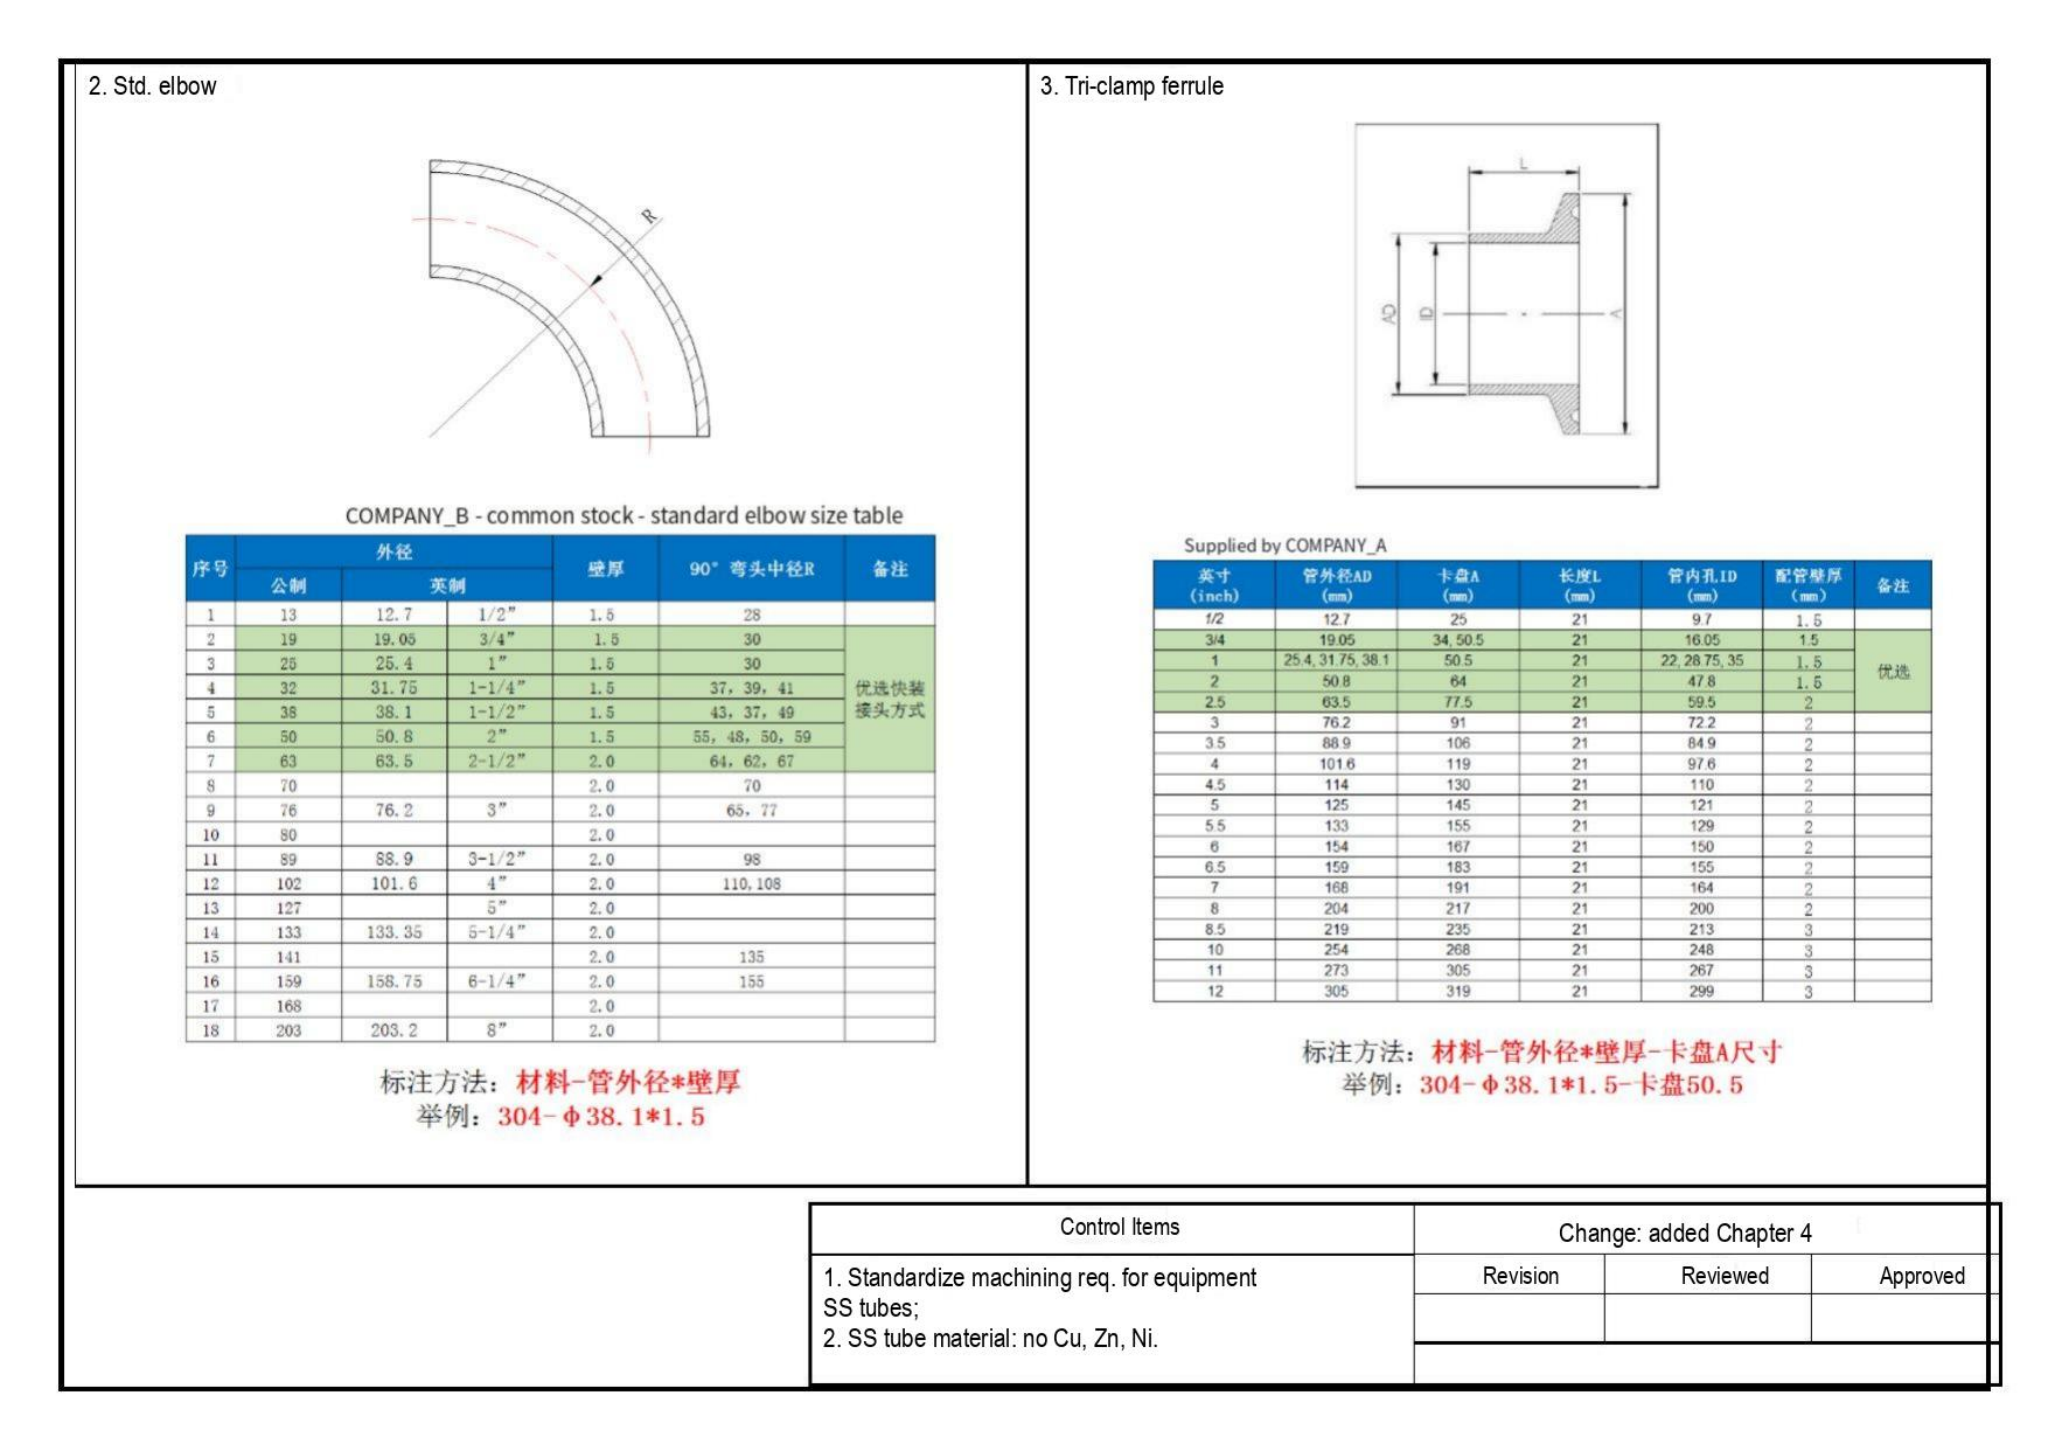2. Std. elbow

R

COMPANY_B - common stock - standard elbow size table

| 序号 | 外径 公制 | 外径 英制 | 外径 英制 | 壁厚 | 90° 弯头中径R | 备注 |
|---|---|---|---|---|---|---|
| 1 | 13 | 12.7 | 1/2" | 1.5 | 28 | |
| 2 | 19 | 19.05 | 3/4" | 1.5 | 30 | 优选快装接头方式 |
| 3 | 25 | 25.4 | 1" | 1.5 | 30 | |
| 4 | 32 | 31.75 | 1-1/4" | 1.5 | 37, 39, 41 | |
| 5 | 38 | 38.1 | 1-1/2" | 1.5 | 43, 37, 49 | |
| 6 | 50 | 50.8 | 2" | 1.5 | 55, 48, 50, 59 | |
| 7 | 63 | 63.5 | 2-1/2" | 2.0 | 64, 62, 67 | |
| 8 | 70 | | | 2.0 | 70 | |
| 9 | 76 | 76.2 | 3" | 2.0 | 65, 77 | |
| 10 | 80 | | | 2.0 | | |
| 11 | 89 | 88.9 | 3-1/2" | 2.0 | 98 | |
| 12 | 102 | 101.6 | 4" | 2.0 | 110, 108 | |
| 13 | 127 | | 5" | 2.0 | | |
| 14 | 133 | 133.35 | 5-1/4" | 2.0 | | |
| 15 | 141 | | | 2.0 | 135 | |
| 16 | 159 | 158.75 | 6-1/4" | 2.0 | 155 | |
| 17 | 168 | | | 2.0 | | |
| 18 | 203 | 203.2 | 8" | 2.0 | | |

标注方法：材料-管外径*壁厚
举例：304-Φ38.1*1.5

3. Tri-clamp ferrule

L
AD
ID
A

Supplied by COMPANY_A

| 英寸 (inch) | 管外径AD (mm) | 卡盘A (mm) | 长度L (mm) | 管内孔ID (mm) | 配管壁厚 (mm) | 备注 |
|---|---|---|---|---|---|---|
| 1/2 | 12.7 | 25 | 21 | 9.7 | 1.5 | |
| 3/4 | 19.05 | 34, 50.5 | 21 | 16.05 | 1.5 | 优选 |
| 1 | 25.4, 31.75, 38.1 | 50.5 | 21 | 22, 28.75, 35 | 1.5 | |
| 2 | 50.8 | 64 | 21 | 47.8 | 1.5 | |
| 2.5 | 63.5 | 77.5 | 21 | 59.5 | 2 | |
| 3 | 76.2 | 91 | 21 | 72.2 | 2 | |
| 3.5 | 88.9 | 106 | 21 | 84.9 | 2 | |
| 4 | 101.6 | 119 | 21 | 97.6 | 2 | |
| 4.5 | 114 | 130 | 21 | 110 | 2 | |
| 5 | 125 | 145 | 21 | 121 | 2 | |
| 5.5 | 133 | 155 | 21 | 129 | 2 | |
| 6 | 154 | 167 | 21 | 150 | 2 | |
| 6.5 | 159 | 183 | 21 | 155 | 2 | |
| 7 | 168 | 191 | 21 | 164 | 2 | |
| 8 | 204 | 217 | 21 | 200 | 2 | |
| 8.5 | 219 | 235 | 21 | 213 | 3 | |
| 10 | 254 | 268 | 21 | 248 | 3 | |
| 11 | 273 | 305 | 21 | 267 | 3 | |
| 12 | 305 | 319 | 21 | 299 | 3 | |

标注方法：材料-管外径*壁厚-卡盘A尺寸
举例：304-Φ38.1*1.5-卡盘50.5

| Control Items | Change: added Chapter 4 | | |
|---|---|---|---|
| 1. Standardize machining req. for equipment SS tubes;<br>2. SS tube material: no Cu, Zn, Ni. | Revision | Reviewed | Approved |
| | | | |
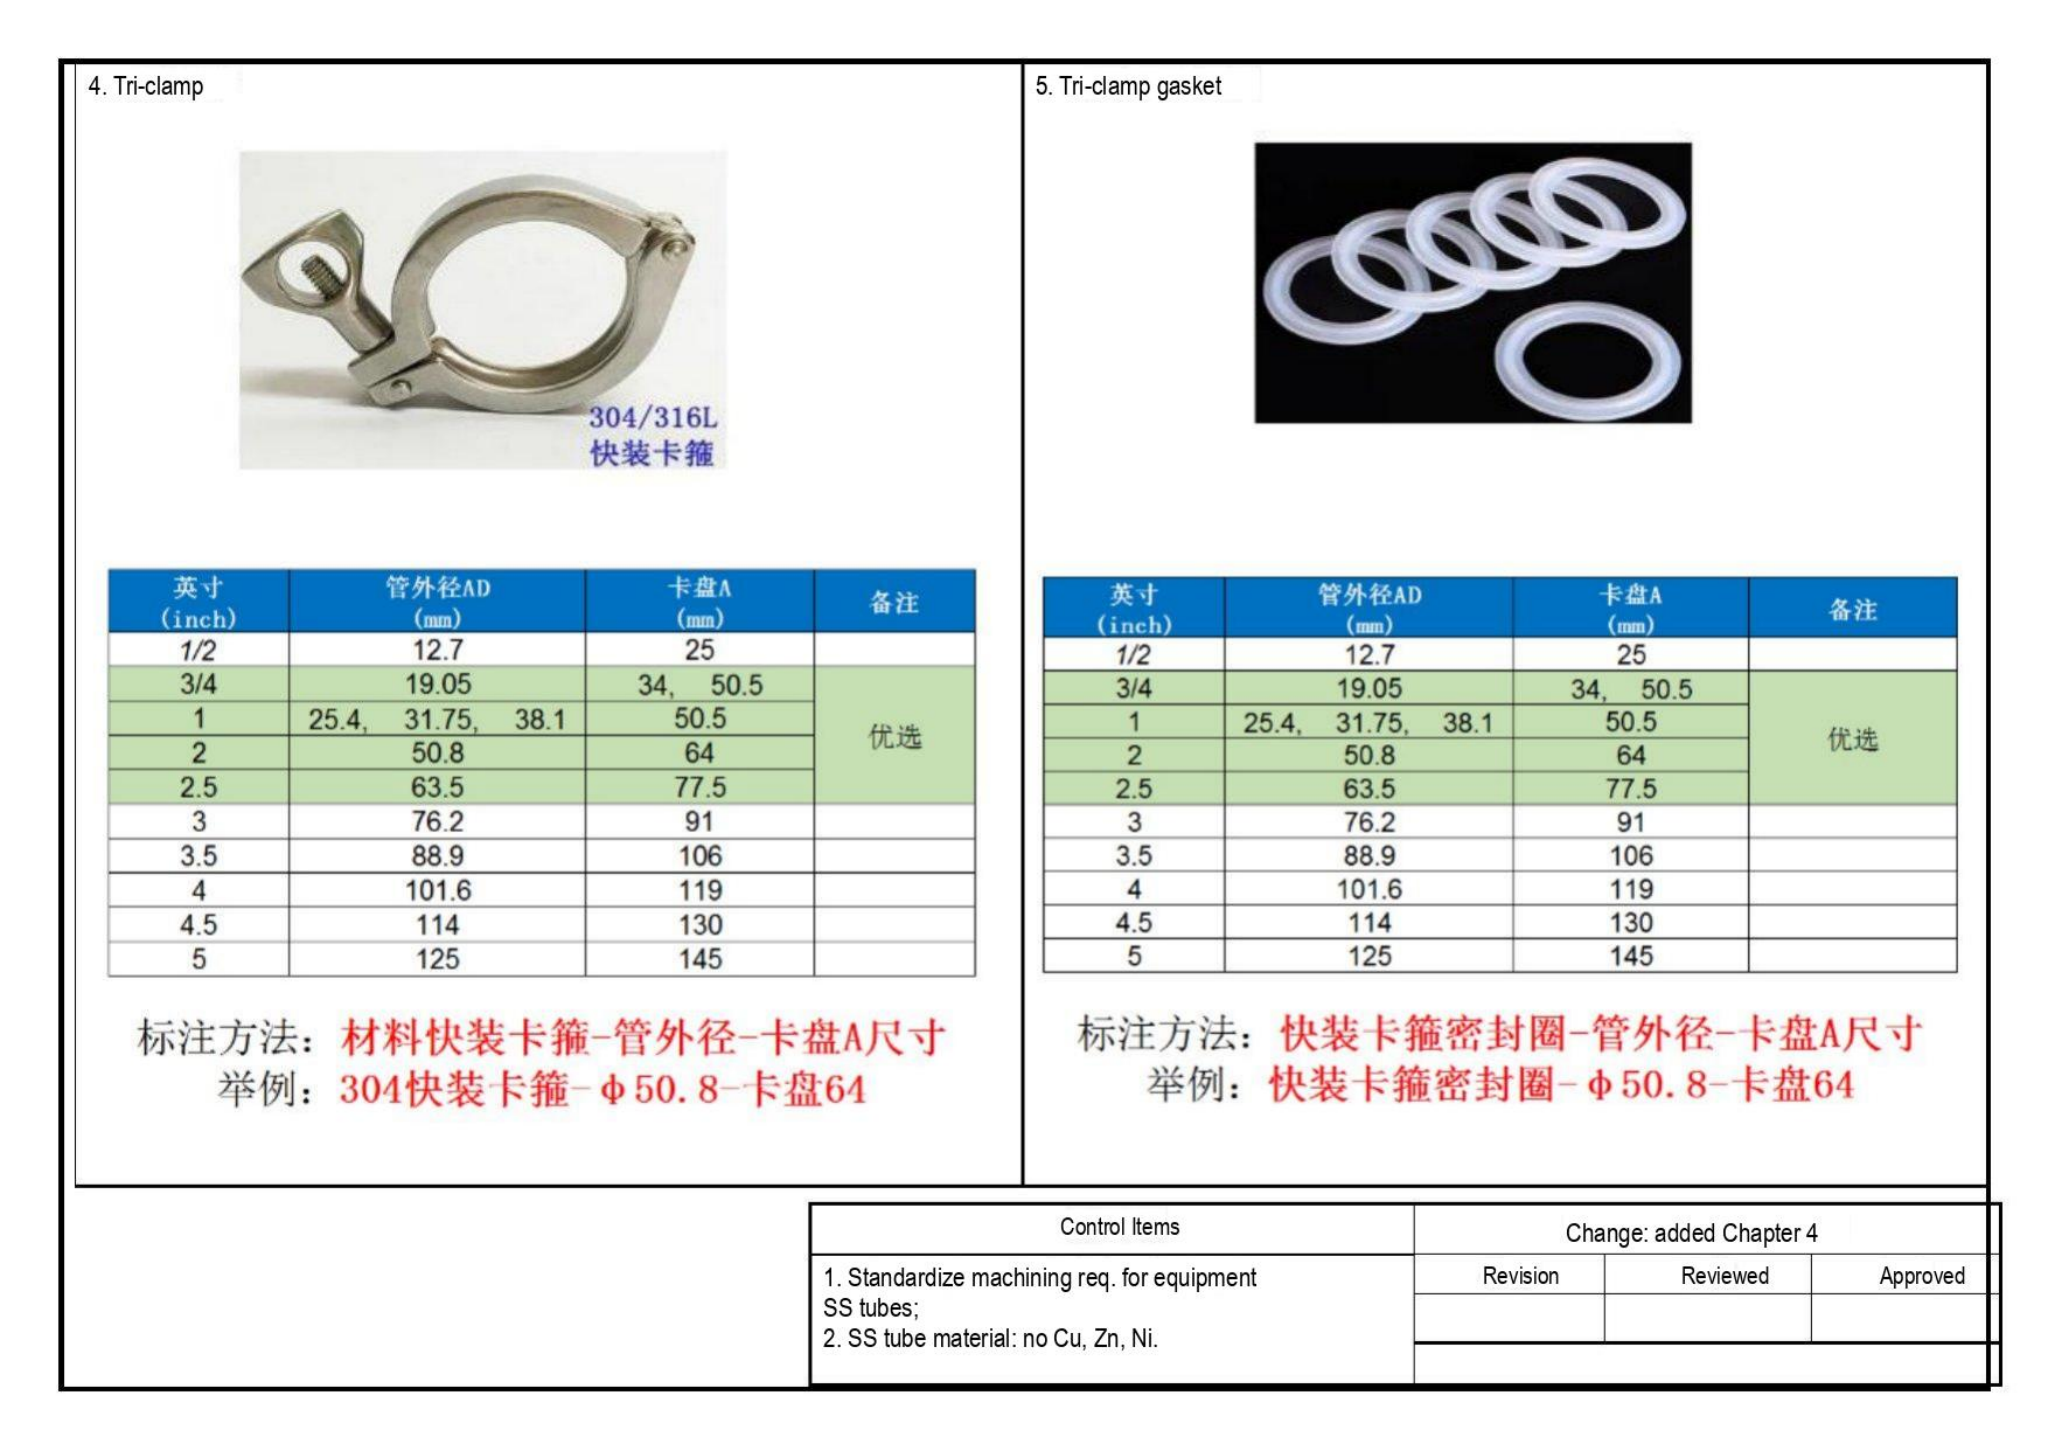4. Tri-clamp

304/316L
快装卡箍

| 英寸 (inch) | 管外径AD (mm) | 卡盘A (mm) | 备注 |
|---|---|---|---|
| 1/2 | 12.7 | 25 | |
| 3/4 | 19.05 | 34, 50.5 | 优选 |
| 1 | 25.4, 31.75, 38.1 | 50.5 | |
| 2 | 50.8 | 64 | |
| 2.5 | 63.5 | 77.5 | |
| 3 | 76.2 | 91 | |
| 3.5 | 88.9 | 106 | |
| 4 | 101.6 | 119 | |
| 4.5 | 114 | 130 | |
| 5 | 125 | 145 | |

标注方法：材料快装卡箍-管外径-卡盘A尺寸
举例：304快装卡箍-φ50.8-卡盘64

5. Tri-clamp gasket

| 英寸 (inch) | 管外径AD (mm) | 卡盘A (mm) | 备注 |
|---|---|---|---|
| 1/2 | 12.7 | 25 | |
| 3/4 | 19.05 | 34, 50.5 | 优选 |
| 1 | 25.4, 31.75, 38.1 | 50.5 | |
| 2 | 50.8 | 64 | |
| 2.5 | 63.5 | 77.5 | |
| 3 | 76.2 | 91 | |
| 3.5 | 88.9 | 106 | |
| 4 | 101.6 | 119 | |
| 4.5 | 114 | 130 | |
| 5 | 125 | 145 | |

标注方法：快装卡箍密封圈-管外径-卡盘A尺寸
举例：快装卡箍密封圈-φ50.8-卡盘64

| Control Items | Change: added Chapter 4 | | |
|---|---|---|---|
| 1. Standardize machining req. for equipment SS tubes;<br>2. SS tube material: no Cu, Zn, Ni. | Revision | Reviewed | Approved |
| | | | |
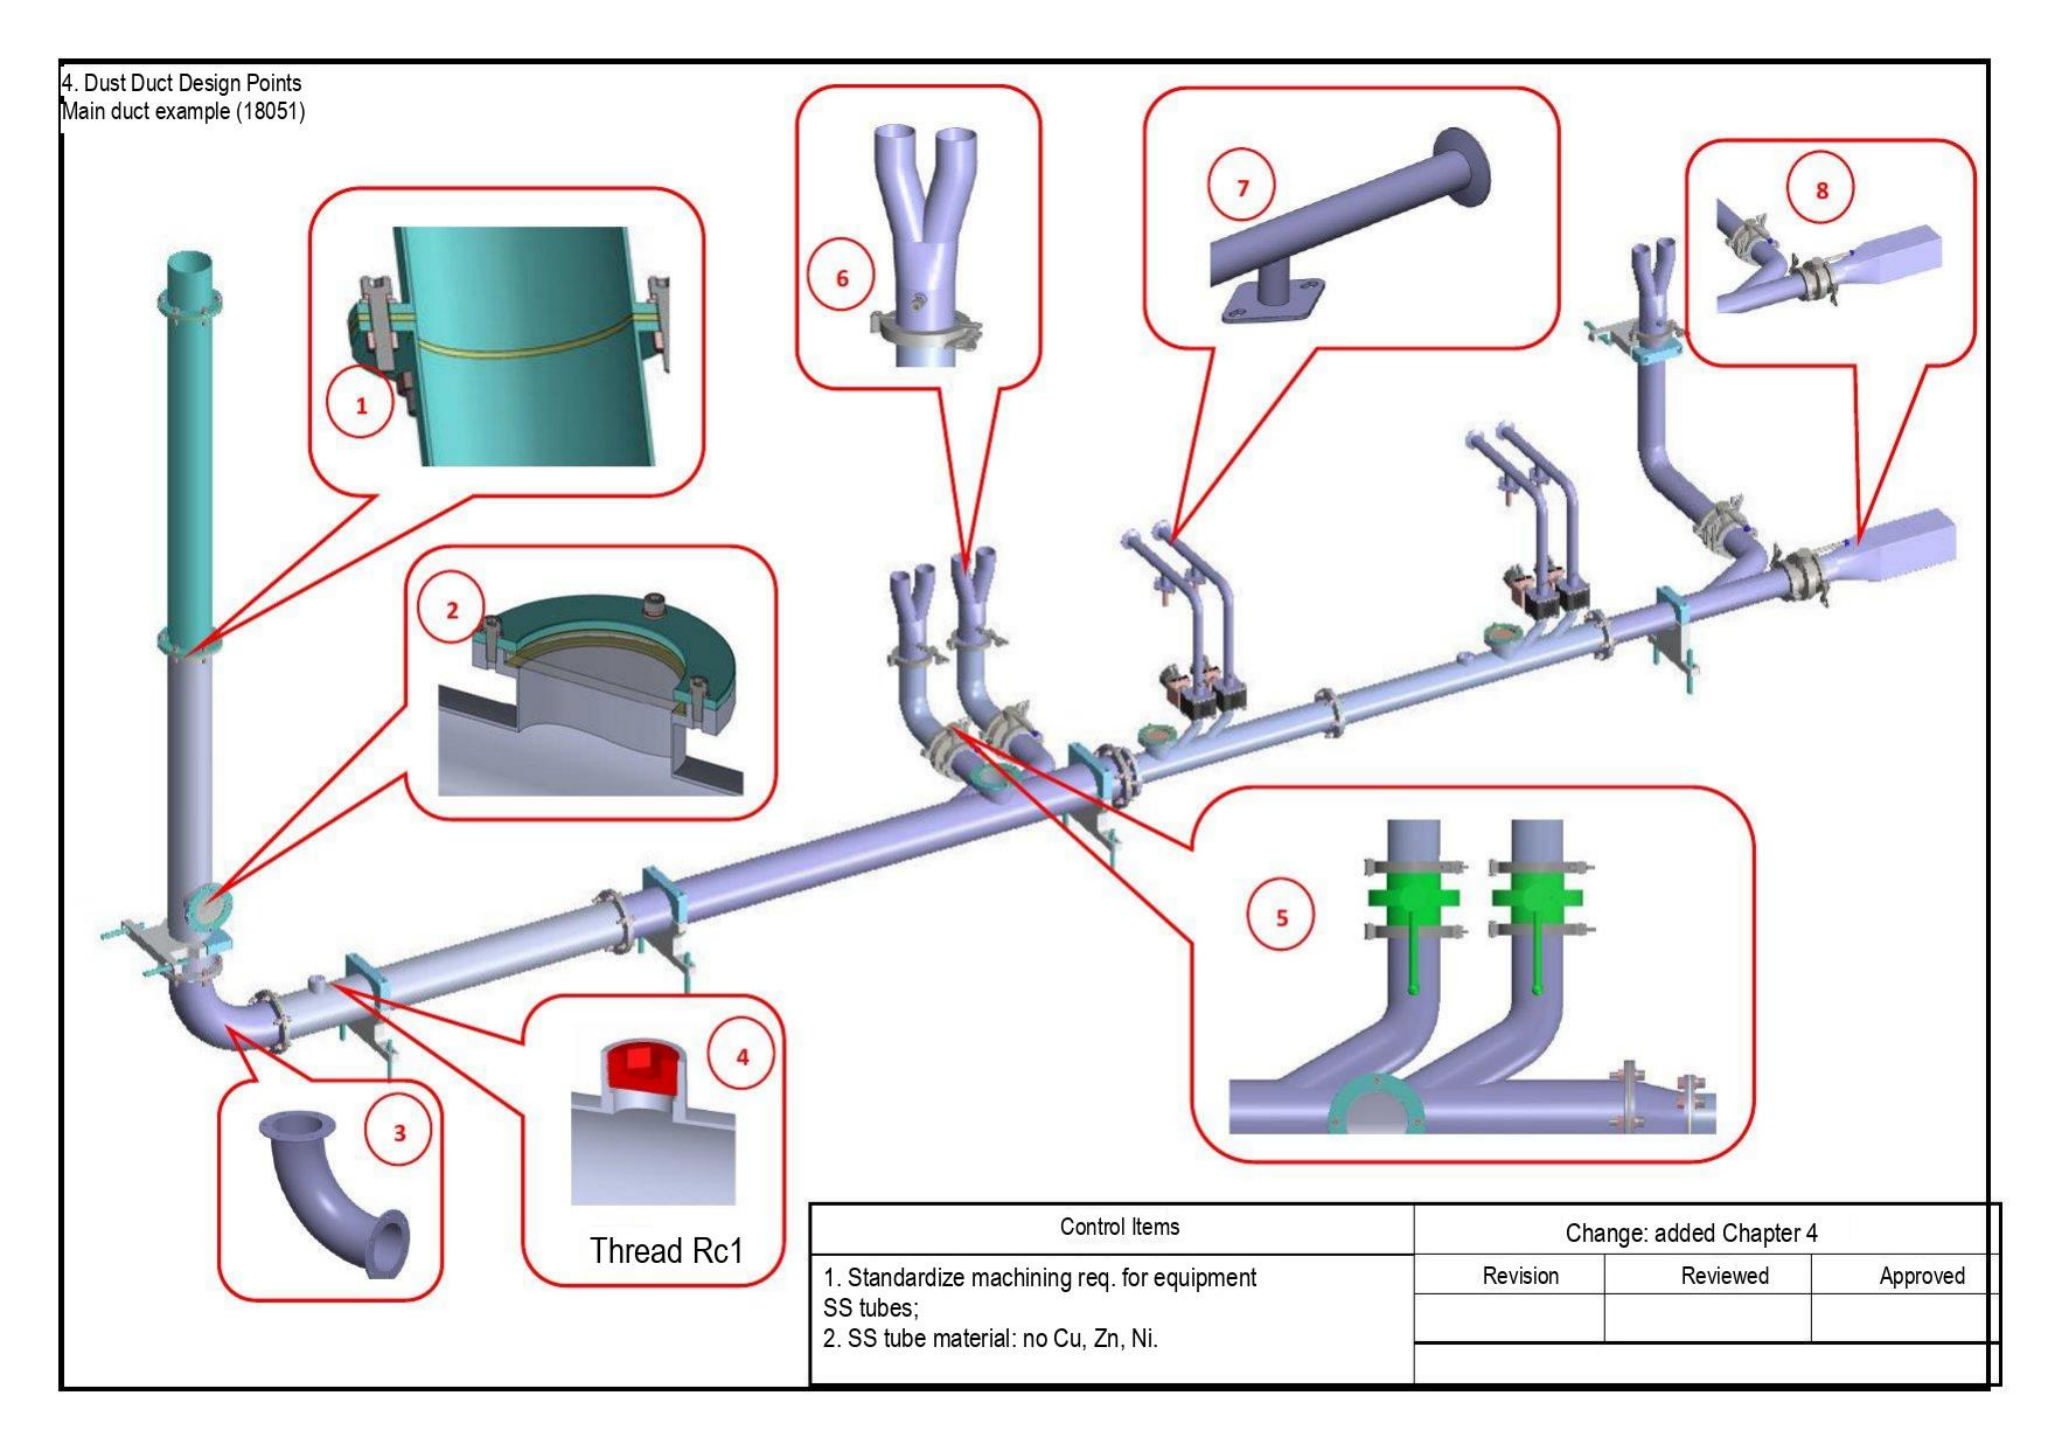4. Dust Duct Design Points
Main duct example (18051)

1

6

7

8

2

5

4

3

Thread Rc1

| Control Items | Change: added Chapter 4 | | |
|---|---|---|---|
| 1. Standardize machining req. for equipment SS tubes;<br>2. SS tube material: no Cu, Zn, Ni. | Revision | Reviewed | Approved |
| | | | |
| | | | |
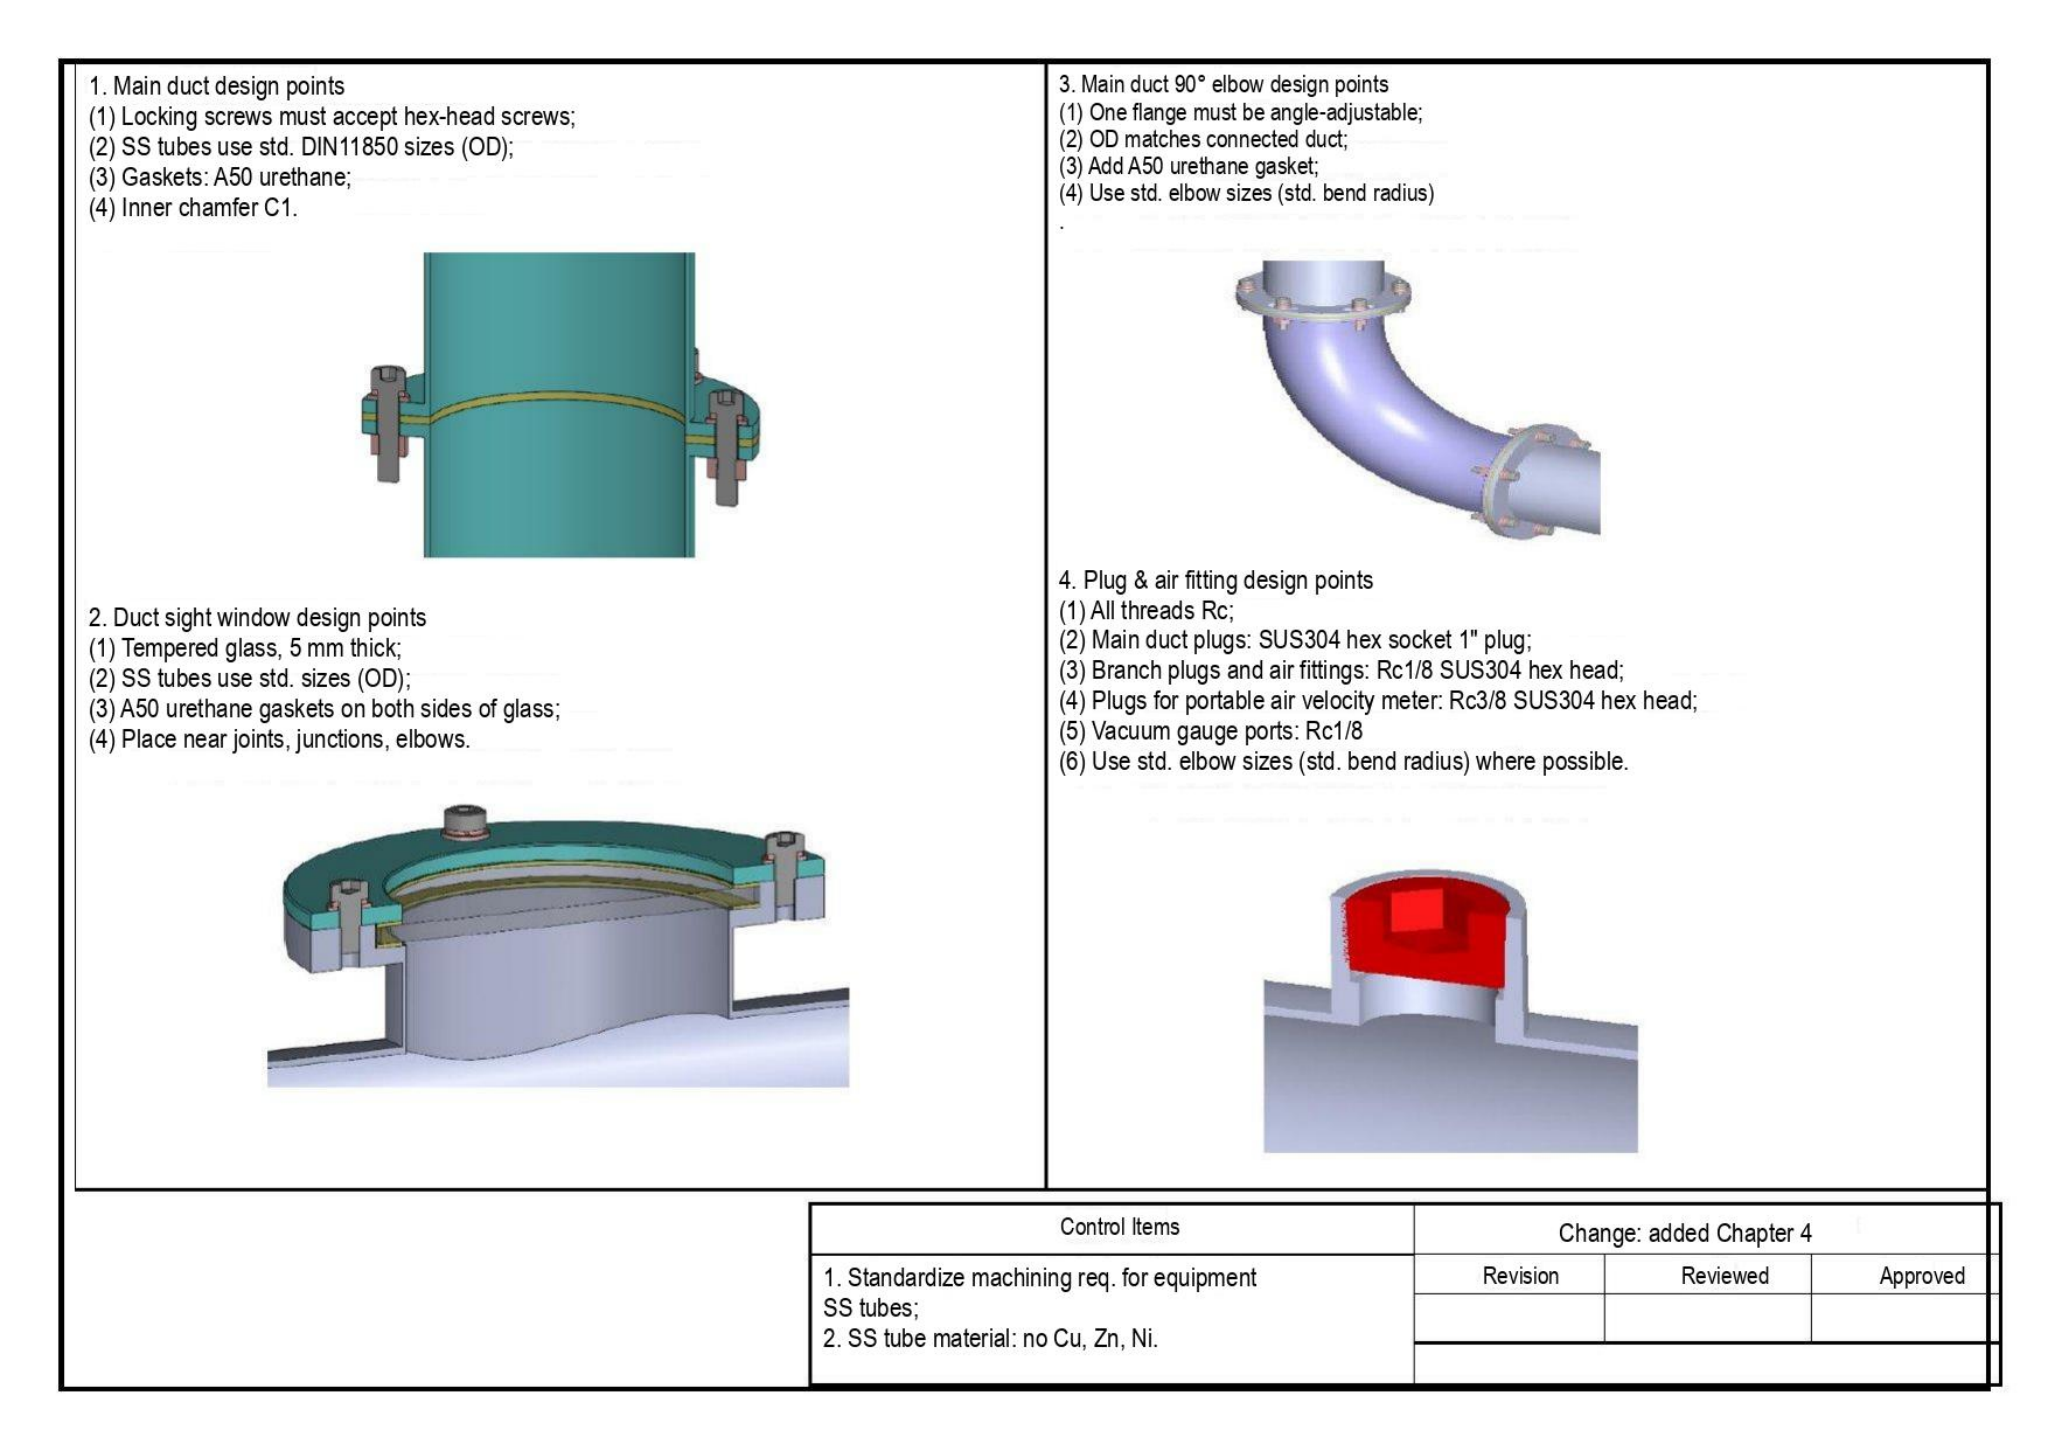1. Main duct design points
(1) Locking screws must accept hex-head screws;
(2) SS tubes use std. DIN11850 sizes (OD);
(3) Gaskets: A50 urethane;
(4) Inner chamfer C1.

2. Duct sight window design points
(1) Tempered glass, 5 mm thick;
(2) SS tubes use std. sizes (OD);
(3) A50 urethane gaskets on both sides of glass;
(4) Place near joints, junctions, elbows.

3. Main duct 90° elbow design points
(1) One flange must be angle-adjustable;
(2) OD matches connected duct;
(3) Add A50 urethane gasket;
(4) Use std. elbow sizes (std. bend radius)
.

4. Plug & air fitting design points
(1) All threads Rc;
(2) Main duct plugs: SUS304 hex socket 1" plug;
(3) Branch plugs and air fittings: Rc1/8 SUS304 hex head;
(4) Plugs for portable air velocity meter: Rc3/8 SUS304 hex head;
(5) Vacuum gauge ports: Rc1/8
(6) Use std. elbow sizes (std. bend radius) where possible.

| Control Items | Change: added Chapter 4 | | |
|---|---|---|---|
| 1. Standardize machining req. for equipment SS tubes;<br>2. SS tube material: no Cu, Zn, Ni. | Revision | Reviewed | Approved |
| | | | |
| | | | |
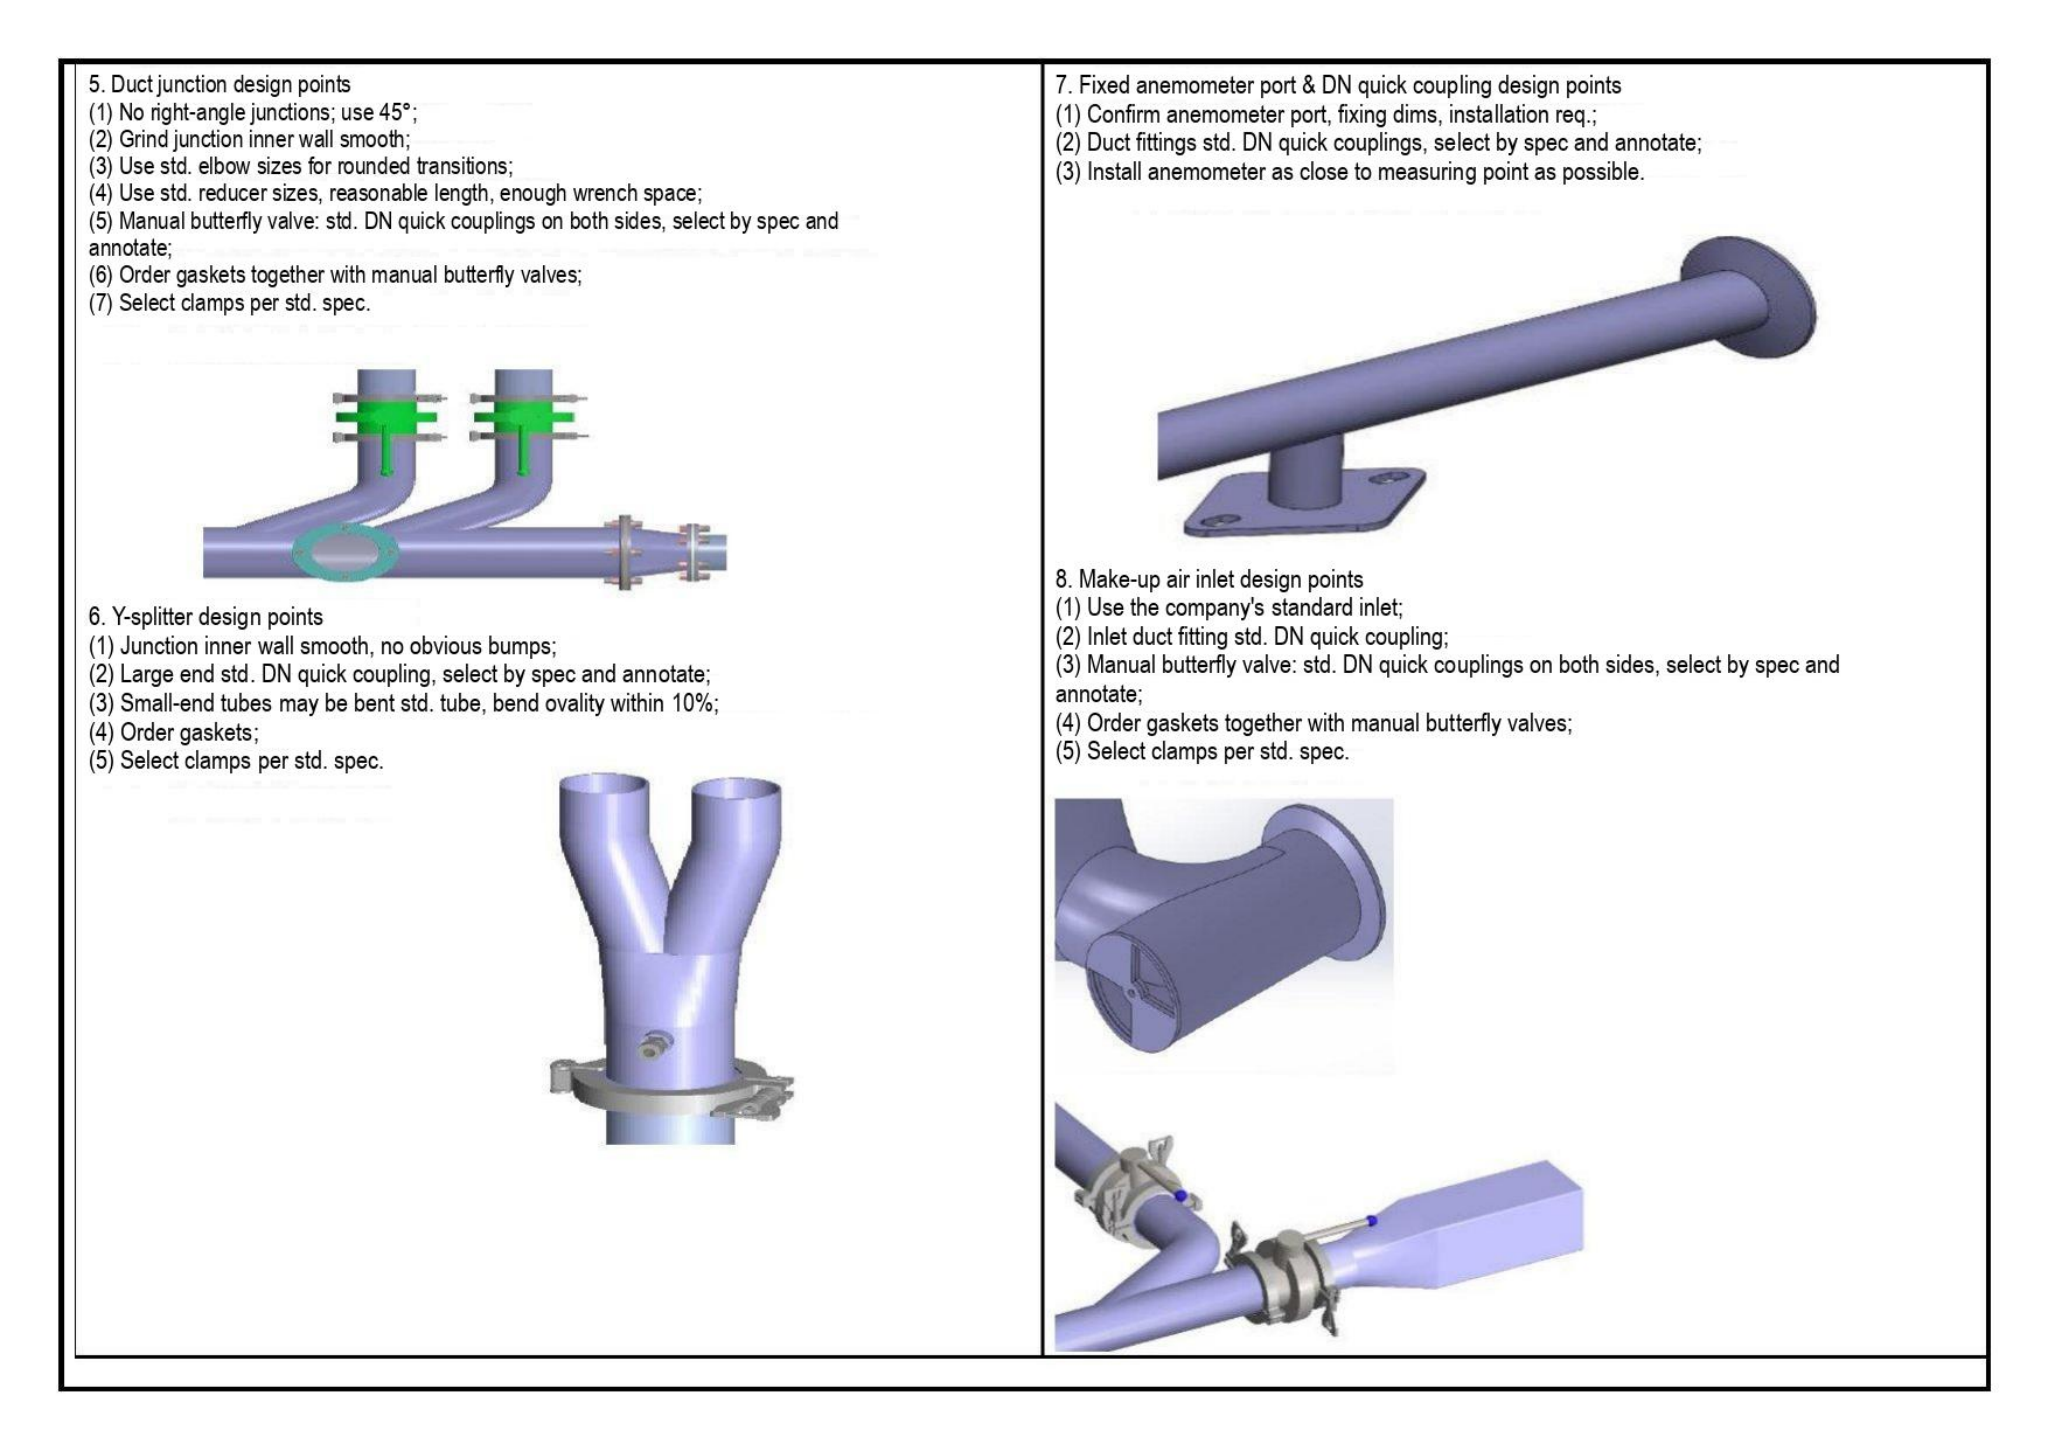5. Duct junction design points
(1) No right-angle junctions; use 45°;
(2) Grind junction inner wall smooth;
(3) Use std. elbow sizes for rounded transitions;
(4) Use std. reducer sizes, reasonable length, enough wrench space;
(5) Manual butterfly valve: std. DN quick couplings on both sides, select by spec and annotate;
(6) Order gaskets together with manual butterfly valves;
(7) Select clamps per std. spec.

6. Y-splitter design points
(1) Junction inner wall smooth, no obvious bumps;
(2) Large end std. DN quick coupling, select by spec and annotate;
(3) Small-end tubes may be bent std. tube, bend ovality within 10%;
(4) Order gaskets;
(5) Select clamps per std. spec.

7. Fixed anemometer port & DN quick coupling design points
(1) Confirm anemometer port, fixing dims, installation req.;
(2) Duct fittings std. DN quick couplings, select by spec and annotate;
(3) Install anemometer as close to measuring point as possible.

8. Make-up air inlet design points
(1) Use the company's standard inlet;
(2) Inlet duct fitting std. DN quick coupling;
(3) Manual butterfly valve: std. DN quick couplings on both sides, select by spec and annotate;
(4) Order gaskets together with manual butterfly valves;
(5) Select clamps per std. spec.
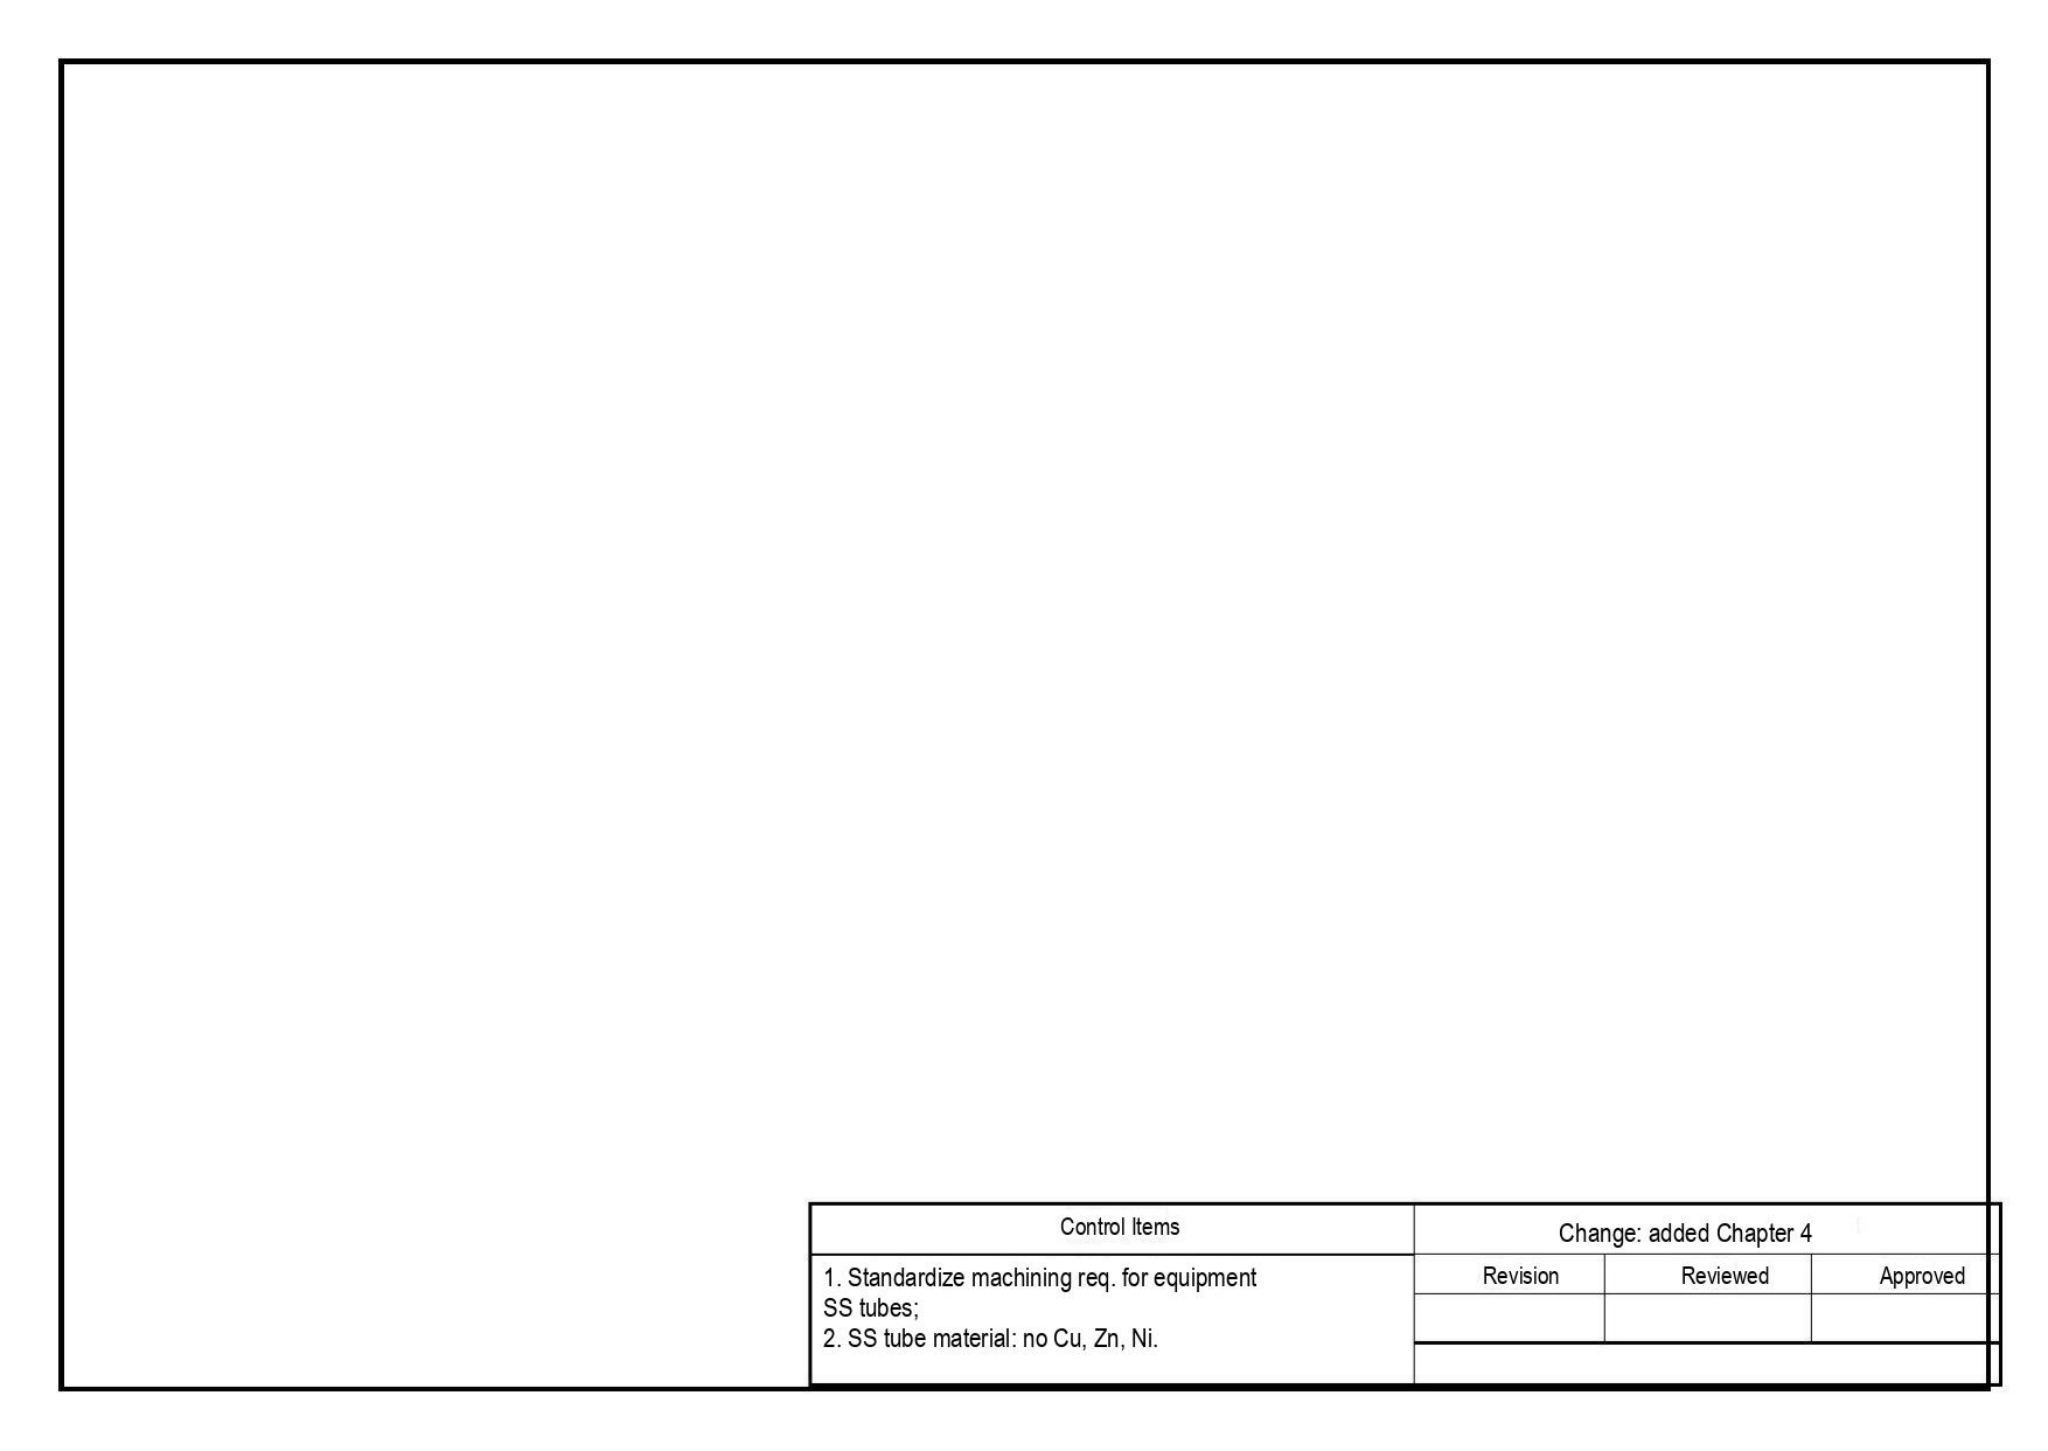| Control Items | Change: added Chapter 4 | | |
|---|---|---|---|
| 1. Standardize machining req. for equipment SS tubes;<br>2. SS tube material: no Cu, Zn, Ni. | Revision | Reviewed | Approved |
| | | | |
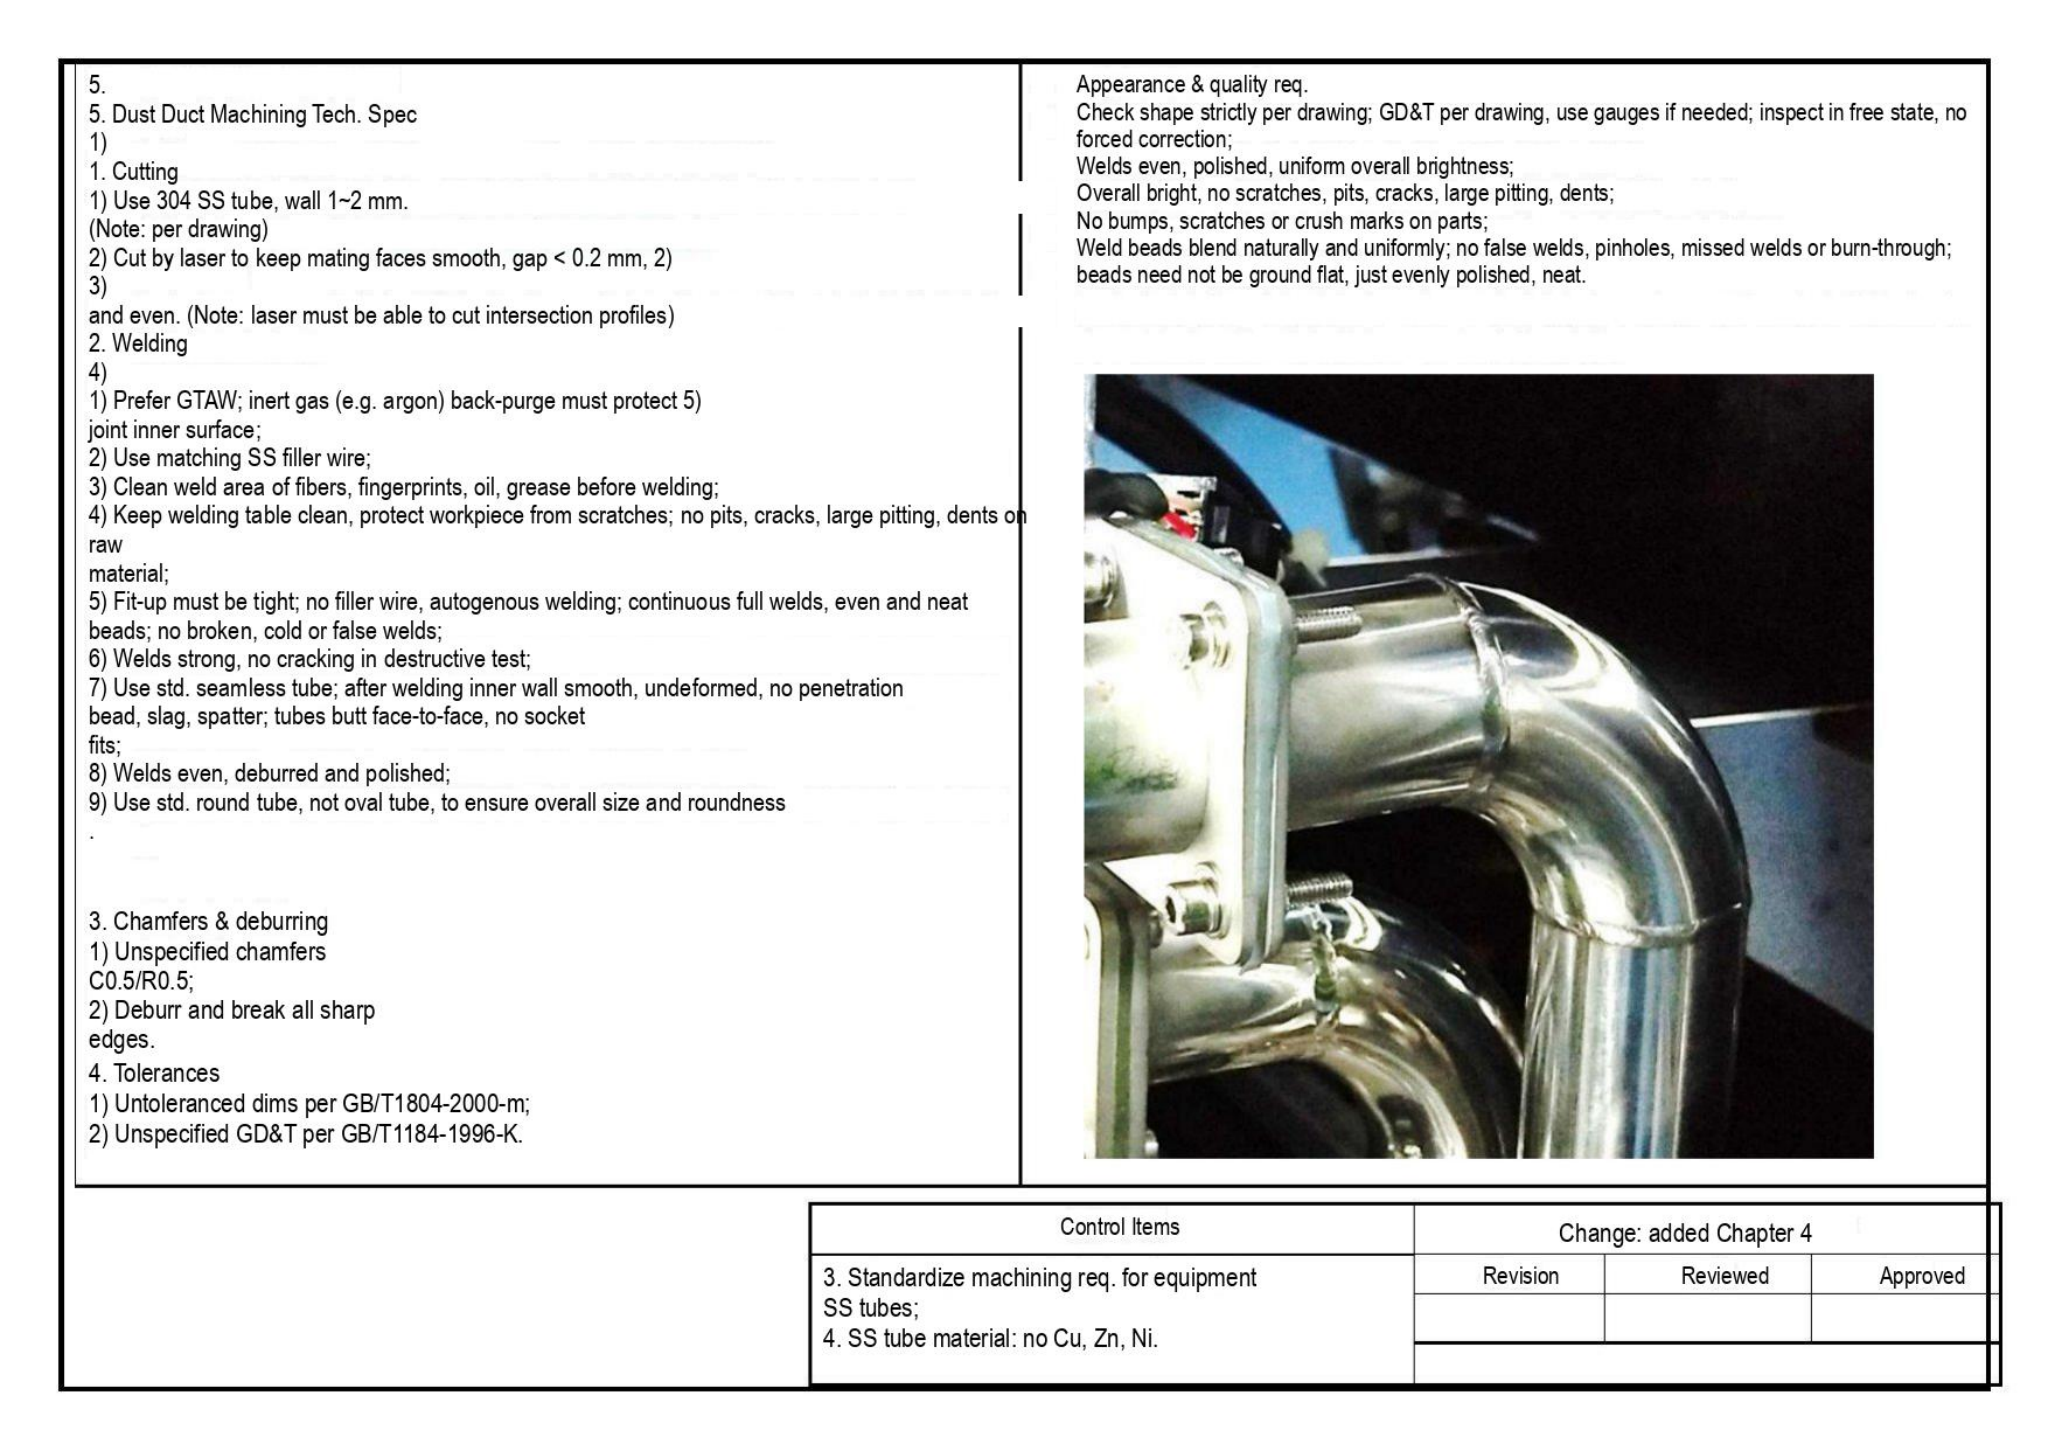5.
5. Dust Duct Machining Tech. Spec
1)
1. Cutting
1) Use 304 SS tube, wall 1~2 mm.
(Note: per drawing)
2) Cut by laser to keep mating faces smooth, gap < 0.2 mm, 2)
3)
and even. (Note: laser must be able to cut intersection profiles)
2. Welding
4)
1) Prefer GTAW; inert gas (e.g. argon) back-purge must protect 5)
joint inner surface;
2) Use matching SS filler wire;
3) Clean weld area of fibers, fingerprints, oil, grease before welding;
4) Keep welding table clean, protect workpiece from scratches; no pits, cracks, large pitting, dents on raw
material;
5) Fit-up must be tight; no filler wire, autogenous welding; continuous full welds, even and neat beads; no broken, cold or false welds;
6) Welds strong, no cracking in destructive test;
7) Use std. seamless tube; after welding inner wall smooth, undeformed, no penetration bead, slag, spatter; tubes butt face-to-face, no socket
fits;
8) Welds even, deburred and polished;
9) Use std. round tube, not oval tube, to ensure overall size and roundness
.

3. Chamfers & deburring
1) Unspecified chamfers
C0.5/R0.5;
2) Deburr and break all sharp
edges.
4. Tolerances
1) Untoleranced dims per GB/T1804-2000-m;
2) Unspecified GD&T per GB/T1184-1996-K.

Appearance & quality req.
Check shape strictly per drawing; GD&T per drawing, use gauges if needed; inspect in free state, no forced correction;
Welds even, polished, uniform overall brightness;
Overall bright, no scratches, pits, cracks, large pitting, dents;
No bumps, scratches or crush marks on parts;
Weld beads blend naturally and uniformly; no false welds, pinholes, missed welds or burn-through; beads need not be ground flat, just evenly polished, neat.

| Control Items | Change: added Chapter 4 | | |
|---|---|---|---|
| 3. Standardize machining req. for equipment SS tubes;<br>4. SS tube material: no Cu, Zn, Ni. | Revision | Reviewed | Approved |
| | | | |